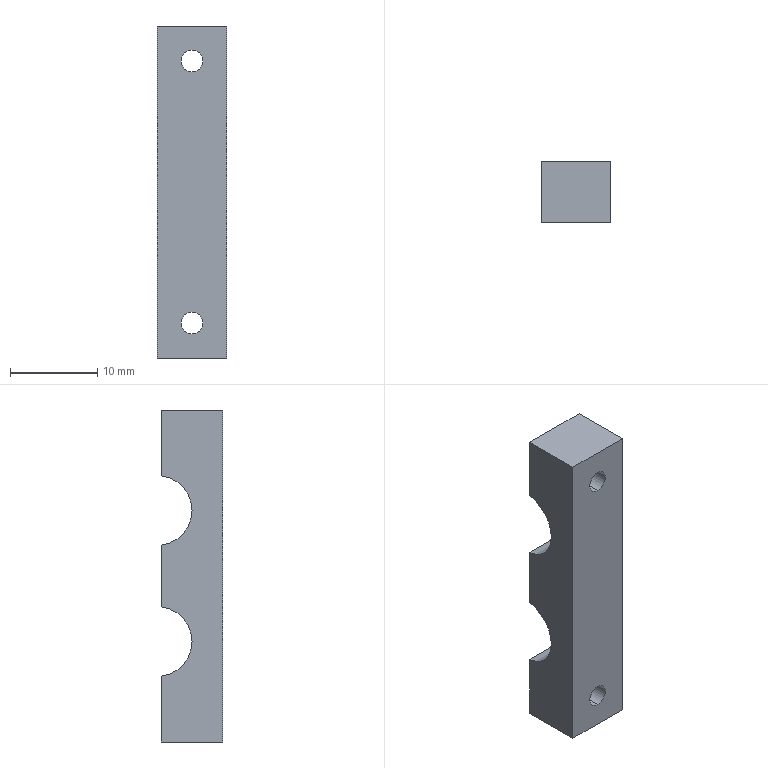Part | STEP file | 0246_217_Block | 1 solid | 14 faces | box 8 x 7 x 38 mm | volume 1721 mm3 | plane 8 | cylinder 6 | commonest cylinder face diameters 2.5 x4 8 x2
STEP:
#1=CARTESIAN_POINT('',(0.,0.,0.));
#2=DIRECTION('',(0.,0.,1.));
#3=DIRECTION('',(1.,0.,0.));
#4=AXIS2_PLACEMENT_3D('',#1,#2,#3);
#5=CARTESIAN_POINT('',(0.,0.,16.25));
#6=VERTEX_POINT('',#5);
#7=CARTESIAN_POINT('',(0.,7.,16.25));
#8=VERTEX_POINT('',#7);
#9=CARTESIAN_POINT('',(0.,7.,16.25));
#10=DIRECTION('',(0.,1.,0.));
#11=VECTOR('',#10,1.);
#12=LINE('',#9,#11);
#13=CARTESIAN_POINT('',(0.,7.,15.));
#14=DIRECTION('',(0.,1.,0.));
#15=DIRECTION('',(0.,0.,1.));
#16=AXIS2_PLACEMENT_3D('',#13,#14,#15);
#17=CYLINDRICAL_SURFACE('',#16,1.25);
#18=CARTESIAN_POINT('',(6.283,0.));
#19=DIRECTION('',(0.,1.));
#20=VECTOR('',#19,1.);
#21=LINE('',#18,#20);
#22=(GEOMETRIC_REPRESENTATION_CONTEXT(2)PARAMETRIC_REPRESENTATION_CONTEXT()REPRESENTATION_CONTEXT('',''));
#23=DEFINITIONAL_REPRESENTATION('',(#21),#22);
#24=PCURVE('',#17,#23);
#25=CARTESIAN_POINT('',(0.,7.,15.));
#26=DIRECTION('',(0.,1.,0.));
#27=DIRECTION('',(0.,0.,1.));
#28=AXIS2_PLACEMENT_3D('',#25,#26,#27);
#29=CYLINDRICAL_SURFACE('',#28,1.25);
#30=CARTESIAN_POINT('',(0.,0.));
#31=DIRECTION('',(0.,1.));
#32=VECTOR('',#31,1.);
#33=LINE('',#30,#32);
#34=(GEOMETRIC_REPRESENTATION_CONTEXT(2)PARAMETRIC_REPRESENTATION_CONTEXT()REPRESENTATION_CONTEXT('',''));
#35=DEFINITIONAL_REPRESENTATION('',(#33),#34);
#36=PCURVE('',#29,#35);
#37=SURFACE_CURVE('',#12,(#24,#36),.PCURVE_S1.);
#38=EDGE_CURVE('',#6,#8,#37,.T.);
#39=ORIENTED_EDGE('',*,*,#38,.T.);
#40=CARTESIAN_POINT('',(0.,7.,13.75));
#41=VERTEX_POINT('',#40);
#42=CARTESIAN_POINT('',(0.,7.,15.));
#43=DIRECTION('',(0.,1.,0.));
#44=DIRECTION('',(0.,0.,1.));
#45=AXIS2_PLACEMENT_3D('',#42,#43,#44);
#46=CIRCLE('',#45,1.25);
#47=CARTESIAN_POINT('',(0.,0.));
#48=DIRECTION('',(1.,0.));
#49=VECTOR('',#48,1.);
#50=LINE('',#47,#49);
#51=(GEOMETRIC_REPRESENTATION_CONTEXT(2)PARAMETRIC_REPRESENTATION_CONTEXT()REPRESENTATION_CONTEXT('',''));
#52=DEFINITIONAL_REPRESENTATION('',(#50),#51);
#53=PCURVE('',#17,#52);
#54=CARTESIAN_POINT('',(4.,7.,19.));
#55=DIRECTION('',(0.,-1.,0.));
#56=DIRECTION('',(0.,0.,-1.));
#57=AXIS2_PLACEMENT_3D('',#54,#55,#56);
#58=PLANE('',#57);
#59=CARTESIAN_POINT('',(2.75,-4.));
#60=CARTESIAN_POINT('',(2.75,-1.835));
#61=CARTESIAN_POINT('',(4.625,-2.917));
#62=CARTESIAN_POINT('',(6.5,-4.));
#63=CARTESIAN_POINT('',(4.625,-5.083));
#64=CARTESIAN_POINT('',(2.75,-6.165));
#65=CARTESIAN_POINT('',(2.75,-4.));
#66=(BOUNDED_CURVE()B_SPLINE_CURVE(2,(#59,#60,#61,#62,#63,#64,#65),.UNSPECIFIED.,.T.,.F.)B_SPLINE_CURVE_WITH_KNOTS((1,2,2,2,2,1),(-2.094,0.,2.094,4.189,6.283,8.378),.UNSPECIFIED.)CURVE()GEOMETRIC_REPRESENTATION_ITEM()RATIONAL_B_SPLINE_CURVE((1.,0.5,1.,0.5,1.,0.5,1.))REPRESENTATION_ITEM(''));
#67=(GEOMETRIC_REPRESENTATION_CONTEXT(2)PARAMETRIC_REPRESENTATION_CONTEXT()REPRESENTATION_CONTEXT('',''));
#68=DEFINITIONAL_REPRESENTATION('',(#66),#67);
#69=PCURVE('',#58,#68);
#70=SURFACE_CURVE('',#46,(#53,#69),.PCURVE_S1.);
#71=EDGE_CURVE('',#41,#8,#70,.T.);
#72=ORIENTED_EDGE('',*,*,#71,.F.);
#73=CARTESIAN_POINT('',(0.,0.,13.75));
#74=VERTEX_POINT('',#73);
#75=CARTESIAN_POINT('',(0.,7.,13.75));
#76=DIRECTION('',(0.,1.,0.));
#77=VECTOR('',#76,1.);
#78=LINE('',#75,#77);
#79=CARTESIAN_POINT('',(3.142,0.));
#80=DIRECTION('',(0.,1.));
#81=VECTOR('',#80,1.);
#82=LINE('',#79,#81);
#83=(GEOMETRIC_REPRESENTATION_CONTEXT(2)PARAMETRIC_REPRESENTATION_CONTEXT()REPRESENTATION_CONTEXT('',''));
#84=DEFINITIONAL_REPRESENTATION('',(#82),#83);
#85=PCURVE('',#17,#84);
#86=CARTESIAN_POINT('',(3.142,0.));
#87=DIRECTION('',(0.,1.));
#88=VECTOR('',#87,1.);
#89=LINE('',#86,#88);
#90=(GEOMETRIC_REPRESENTATION_CONTEXT(2)PARAMETRIC_REPRESENTATION_CONTEXT()REPRESENTATION_CONTEXT('',''));
#91=DEFINITIONAL_REPRESENTATION('',(#89),#90);
#92=PCURVE('',#29,#91);
#93=SURFACE_CURVE('',#78,(#85,#92),.PCURVE_S1.);
#94=EDGE_CURVE('',#74,#41,#93,.T.);
#95=ORIENTED_EDGE('',*,*,#94,.F.);
#96=CARTESIAN_POINT('',(0.,0.,15.));
#97=DIRECTION('',(0.,1.,0.));
#98=DIRECTION('',(0.,0.,1.));
#99=AXIS2_PLACEMENT_3D('',#96,#97,#98);
#100=CIRCLE('',#99,1.25);
#101=CARTESIAN_POINT('',(0.,-7.));
#102=DIRECTION('',(1.,0.));
#103=VECTOR('',#102,1.);
#104=LINE('',#101,#103);
#105=(GEOMETRIC_REPRESENTATION_CONTEXT(2)PARAMETRIC_REPRESENTATION_CONTEXT()REPRESENTATION_CONTEXT('',''));
#106=DEFINITIONAL_REPRESENTATION('',(#104),#105);
#107=PCURVE('',#17,#106);
#108=CARTESIAN_POINT('',(4.,0.,19.));
#109=DIRECTION('',(0.,1.,0.));
#110=DIRECTION('',(0.,0.,1.));
#111=AXIS2_PLACEMENT_3D('',#108,#109,#110);
#112=PLANE('',#111);
#113=CARTESIAN_POINT('',(-4.,-4.));
#114=DIRECTION('',(1.,0.));
#115=AXIS2_PLACEMENT_2D('',#113,#114);
#116=CIRCLE('',#115,1.25);
#117=(GEOMETRIC_REPRESENTATION_CONTEXT(2)PARAMETRIC_REPRESENTATION_CONTEXT()REPRESENTATION_CONTEXT('',''));
#118=DEFINITIONAL_REPRESENTATION('',(#116),#117);
#119=PCURVE('',#112,#118);
#120=SURFACE_CURVE('',#100,(#107,#119),.PCURVE_S1.);
#121=EDGE_CURVE('',#74,#6,#120,.T.);
#122=ORIENTED_EDGE('',*,*,#121,.T.);
#123=EDGE_LOOP('',(#39,#72,#95,#122));
#124=FACE_BOUND('',#123,.F.);
#125=ADVANCED_FACE('',(#124),#17,.F.);
#126=CARTESIAN_POINT('',(0.,0.,-13.75));
#127=VERTEX_POINT('',#126);
#128=CARTESIAN_POINT('',(0.,7.,-13.75));
#129=VERTEX_POINT('',#128);
#130=CARTESIAN_POINT('',(0.,7.,-13.75));
#131=DIRECTION('',(0.,1.,0.));
#132=VECTOR('',#131,1.);
#133=LINE('',#130,#132);
#134=CARTESIAN_POINT('',(0.,7.,-15.));
#135=DIRECTION('',(0.,1.,0.));
#136=DIRECTION('',(0.,0.,1.));
#137=AXIS2_PLACEMENT_3D('',#134,#135,#136);
#138=CYLINDRICAL_SURFACE('',#137,1.25);
#139=CARTESIAN_POINT('',(6.283,0.));
#140=DIRECTION('',(0.,1.));
#141=VECTOR('',#140,1.);
#142=LINE('',#139,#141);
#143=(GEOMETRIC_REPRESENTATION_CONTEXT(2)PARAMETRIC_REPRESENTATION_CONTEXT()REPRESENTATION_CONTEXT('',''));
#144=DEFINITIONAL_REPRESENTATION('',(#142),#143);
#145=PCURVE('',#138,#144);
#146=CARTESIAN_POINT('',(0.,7.,-15.));
#147=DIRECTION('',(0.,1.,0.));
#148=DIRECTION('',(0.,0.,1.));
#149=AXIS2_PLACEMENT_3D('',#146,#147,#148);
#150=CYLINDRICAL_SURFACE('',#149,1.25);
#151=CARTESIAN_POINT('',(0.,0.));
#152=DIRECTION('',(0.,1.));
#153=VECTOR('',#152,1.);
#154=LINE('',#151,#153);
#155=(GEOMETRIC_REPRESENTATION_CONTEXT(2)PARAMETRIC_REPRESENTATION_CONTEXT()REPRESENTATION_CONTEXT('',''));
#156=DEFINITIONAL_REPRESENTATION('',(#154),#155);
#157=PCURVE('',#150,#156);
#158=SURFACE_CURVE('',#133,(#145,#157),.PCURVE_S1.);
#159=EDGE_CURVE('',#127,#129,#158,.T.);
#160=ORIENTED_EDGE('',*,*,#159,.T.);
#161=CARTESIAN_POINT('',(0.,7.,-16.25));
#162=VERTEX_POINT('',#161);
#163=CARTESIAN_POINT('',(0.,7.,-15.));
#164=DIRECTION('',(0.,1.,0.));
#165=DIRECTION('',(0.,0.,1.));
#166=AXIS2_PLACEMENT_3D('',#163,#164,#165);
#167=CIRCLE('',#166,1.25);
#168=CARTESIAN_POINT('',(0.,0.));
#169=DIRECTION('',(1.,0.));
#170=VECTOR('',#169,1.);
#171=LINE('',#168,#170);
#172=(GEOMETRIC_REPRESENTATION_CONTEXT(2)PARAMETRIC_REPRESENTATION_CONTEXT()REPRESENTATION_CONTEXT('',''));
#173=DEFINITIONAL_REPRESENTATION('',(#171),#172);
#174=PCURVE('',#138,#173);
#175=CARTESIAN_POINT('',(4.,7.,-19.));
#176=DIRECTION('',(0.,-1.,0.));
#177=DIRECTION('',(0.,0.,-1.));
#178=AXIS2_PLACEMENT_3D('',#175,#176,#177);
#179=PLANE('',#178);
#180=CARTESIAN_POINT('',(-5.25,-4.));
#181=CARTESIAN_POINT('',(-5.25,-1.835));
#182=CARTESIAN_POINT('',(-3.375,-2.917));
#183=CARTESIAN_POINT('',(-1.5,-4.));
#184=CARTESIAN_POINT('',(-3.375,-5.083));
#185=CARTESIAN_POINT('',(-5.25,-6.165));
#186=CARTESIAN_POINT('',(-5.25,-4.));
#187=(BOUNDED_CURVE()B_SPLINE_CURVE(2,(#180,#181,#182,#183,#184,#185,#186),.UNSPECIFIED.,.T.,.F.)B_SPLINE_CURVE_WITH_KNOTS((1,2,2,2,2,1),(-2.094,0.,2.094,4.189,6.283,8.378),.UNSPECIFIED.)CURVE()GEOMETRIC_REPRESENTATION_ITEM()RATIONAL_B_SPLINE_CURVE((1.,0.5,1.,0.5,1.,0.5,1.))REPRESENTATION_ITEM(''));
#188=(GEOMETRIC_REPRESENTATION_CONTEXT(2)PARAMETRIC_REPRESENTATION_CONTEXT()REPRESENTATION_CONTEXT('',''));
#189=DEFINITIONAL_REPRESENTATION('',(#187),#188);
#190=PCURVE('',#179,#189);
#191=SURFACE_CURVE('',#167,(#174,#190),.PCURVE_S1.);
#192=EDGE_CURVE('',#162,#129,#191,.T.);
#193=ORIENTED_EDGE('',*,*,#192,.F.);
#194=CARTESIAN_POINT('',(0.,0.,-16.25));
#195=VERTEX_POINT('',#194);
#196=CARTESIAN_POINT('',(0.,7.,-16.25));
#197=DIRECTION('',(0.,1.,0.));
#198=VECTOR('',#197,1.);
#199=LINE('',#196,#198);
#200=CARTESIAN_POINT('',(3.142,0.));
#201=DIRECTION('',(0.,1.));
#202=VECTOR('',#201,1.);
#203=LINE('',#200,#202);
#204=(GEOMETRIC_REPRESENTATION_CONTEXT(2)PARAMETRIC_REPRESENTATION_CONTEXT()REPRESENTATION_CONTEXT('',''));
#205=DEFINITIONAL_REPRESENTATION('',(#203),#204);
#206=PCURVE('',#138,#205);
#207=CARTESIAN_POINT('',(3.142,0.));
#208=DIRECTION('',(0.,1.));
#209=VECTOR('',#208,1.);
#210=LINE('',#207,#209);
#211=(GEOMETRIC_REPRESENTATION_CONTEXT(2)PARAMETRIC_REPRESENTATION_CONTEXT()REPRESENTATION_CONTEXT('',''));
#212=DEFINITIONAL_REPRESENTATION('',(#210),#211);
#213=PCURVE('',#150,#212);
#214=SURFACE_CURVE('',#199,(#206,#213),.PCURVE_S1.);
#215=EDGE_CURVE('',#195,#162,#214,.T.);
#216=ORIENTED_EDGE('',*,*,#215,.F.);
#217=CARTESIAN_POINT('',(0.,0.,-15.));
#218=DIRECTION('',(0.,1.,0.));
#219=DIRECTION('',(0.,0.,1.));
#220=AXIS2_PLACEMENT_3D('',#217,#218,#219);
#221=CIRCLE('',#220,1.25);
#222=CARTESIAN_POINT('',(0.,-7.));
#223=DIRECTION('',(1.,0.));
#224=VECTOR('',#223,1.);
#225=LINE('',#222,#224);
#226=(GEOMETRIC_REPRESENTATION_CONTEXT(2)PARAMETRIC_REPRESENTATION_CONTEXT()REPRESENTATION_CONTEXT('',''));
#227=DEFINITIONAL_REPRESENTATION('',(#225),#226);
#228=PCURVE('',#138,#227);
#229=CARTESIAN_POINT('',(-34.,-4.));
#230=DIRECTION('',(1.,0.));
#231=AXIS2_PLACEMENT_2D('',#229,#230);
#232=CIRCLE('',#231,1.25);
#233=(GEOMETRIC_REPRESENTATION_CONTEXT(2)PARAMETRIC_REPRESENTATION_CONTEXT()REPRESENTATION_CONTEXT('',''));
#234=DEFINITIONAL_REPRESENTATION('',(#232),#233);
#235=PCURVE('',#112,#234);
#236=SURFACE_CURVE('',#221,(#228,#235),.PCURVE_S1.);
#237=EDGE_CURVE('',#195,#127,#236,.T.);
#238=ORIENTED_EDGE('',*,*,#237,.T.);
#239=EDGE_LOOP('',(#160,#193,#216,#238));
#240=FACE_BOUND('',#239,.F.);
#241=ADVANCED_FACE('',(#240),#138,.F.);
#242=CARTESIAN_POINT('',(-4.,7.,19.));
#243=VERTEX_POINT('',#242);
#244=CARTESIAN_POINT('',(-4.,0.,19.));
#245=VERTEX_POINT('',#244);
#246=CARTESIAN_POINT('',(-4.,0.,19.));
#247=DIRECTION('',(0.,-1.,0.));
#248=VECTOR('',#247,1.);
#249=LINE('',#246,#248);
#250=CARTESIAN_POINT('',(4.,0.,19.));
#251=DIRECTION('',(0.,0.,-1.));
#252=DIRECTION('',(-1.,0.,0.));
#253=AXIS2_PLACEMENT_3D('',#250,#251,#252);
#254=PLANE('',#253);
#255=CARTESIAN_POINT('',(8.,0.));
#256=DIRECTION('',(0.,-1.));
#257=VECTOR('',#256,1.);
#258=LINE('',#255,#257);
#259=(GEOMETRIC_REPRESENTATION_CONTEXT(2)PARAMETRIC_REPRESENTATION_CONTEXT()REPRESENTATION_CONTEXT('',''));
#260=DEFINITIONAL_REPRESENTATION('',(#258),#259);
#261=PCURVE('',#254,#260);
#262=CARTESIAN_POINT('',(-4.,7.5,7.5));
#263=DIRECTION('',(1.,0.,0.));
#264=DIRECTION('',(0.,0.,-1.));
#265=AXIS2_PLACEMENT_3D('',#262,#263,#264);
#266=PLANE('',#265);
#267=CARTESIAN_POINT('',(-11.5,-7.5));
#268=DIRECTION('',(0.,-1.));
#269=VECTOR('',#268,1.);
#270=LINE('',#267,#269);
#271=(GEOMETRIC_REPRESENTATION_CONTEXT(2)PARAMETRIC_REPRESENTATION_CONTEXT()REPRESENTATION_CONTEXT('',''));
#272=DEFINITIONAL_REPRESENTATION('',(#270),#271);
#273=PCURVE('',#266,#272);
#274=SURFACE_CURVE('',#249,(#261,#273),.PCURVE_S1.);
#275=EDGE_CURVE('',#243,#245,#274,.T.);
#276=ORIENTED_EDGE('',*,*,#275,.T.);
#277=CARTESIAN_POINT('',(4.,0.,19.));
#278=VERTEX_POINT('',#277);
#279=CARTESIAN_POINT('',(4.,0.,19.));
#280=DIRECTION('',(-1.,0.,0.));
#281=VECTOR('',#280,1.);
#282=LINE('',#279,#281);
#283=CARTESIAN_POINT('',(0.,0.));
#284=DIRECTION('',(1.,0.));
#285=VECTOR('',#284,1.);
#286=LINE('',#283,#285);
#287=(GEOMETRIC_REPRESENTATION_CONTEXT(2)PARAMETRIC_REPRESENTATION_CONTEXT()REPRESENTATION_CONTEXT('',''));
#288=DEFINITIONAL_REPRESENTATION('',(#286),#287);
#289=PCURVE('',#254,#288);
#290=CARTESIAN_POINT('',(0.,0.));
#291=DIRECTION('',(0.,-1.));
#292=VECTOR('',#291,1.);
#293=LINE('',#290,#292);
#294=(GEOMETRIC_REPRESENTATION_CONTEXT(2)PARAMETRIC_REPRESENTATION_CONTEXT()REPRESENTATION_CONTEXT('',''));
#295=DEFINITIONAL_REPRESENTATION('',(#293),#294);
#296=PCURVE('',#112,#295);
#297=SURFACE_CURVE('',#282,(#289,#296),.PCURVE_S1.);
#298=EDGE_CURVE('',#278,#245,#297,.T.);
#299=ORIENTED_EDGE('',*,*,#298,.F.);
#300=CARTESIAN_POINT('',(4.,7.,19.));
#301=VERTEX_POINT('',#300);
#302=CARTESIAN_POINT('',(4.,0.,19.));
#303=DIRECTION('',(0.,-1.,0.));
#304=VECTOR('',#303,1.);
#305=LINE('',#302,#304);
#306=CARTESIAN_POINT('',(0.,0.));
#307=DIRECTION('',(0.,-1.));
#308=VECTOR('',#307,1.);
#309=LINE('',#306,#308);
#310=(GEOMETRIC_REPRESENTATION_CONTEXT(2)PARAMETRIC_REPRESENTATION_CONTEXT()REPRESENTATION_CONTEXT('',''));
#311=DEFINITIONAL_REPRESENTATION('',(#309),#310);
#312=PCURVE('',#254,#311);
#313=CARTESIAN_POINT('',(4.,7.5,7.5));
#314=DIRECTION('',(1.,0.,0.));
#315=DIRECTION('',(0.,0.,-1.));
#316=AXIS2_PLACEMENT_3D('',#313,#314,#315);
#317=PLANE('',#316);
#318=CARTESIAN_POINT('',(-11.5,-7.5));
#319=DIRECTION('',(0.,-1.));
#320=VECTOR('',#319,1.);
#321=LINE('',#318,#320);
#322=(GEOMETRIC_REPRESENTATION_CONTEXT(2)PARAMETRIC_REPRESENTATION_CONTEXT()REPRESENTATION_CONTEXT('',''));
#323=DEFINITIONAL_REPRESENTATION('',(#321),#322);
#324=PCURVE('',#317,#323);
#325=SURFACE_CURVE('',#305,(#312,#324),.PCURVE_S1.);
#326=EDGE_CURVE('',#301,#278,#325,.T.);
#327=ORIENTED_EDGE('',*,*,#326,.F.);
#328=CARTESIAN_POINT('',(4.,7.,19.));
#329=DIRECTION('',(-1.,0.,0.));
#330=VECTOR('',#329,1.);
#331=LINE('',#328,#330);
#332=CARTESIAN_POINT('',(0.,7.));
#333=DIRECTION('',(1.,0.));
#334=VECTOR('',#333,1.);
#335=LINE('',#332,#334);
#336=(GEOMETRIC_REPRESENTATION_CONTEXT(2)PARAMETRIC_REPRESENTATION_CONTEXT()REPRESENTATION_CONTEXT('',''));
#337=DEFINITIONAL_REPRESENTATION('',(#335),#336);
#338=PCURVE('',#254,#337);
#339=CARTESIAN_POINT('',(0.,0.));
#340=DIRECTION('',(0.,-1.));
#341=VECTOR('',#340,1.);
#342=LINE('',#339,#341);
#343=(GEOMETRIC_REPRESENTATION_CONTEXT(2)PARAMETRIC_REPRESENTATION_CONTEXT()REPRESENTATION_CONTEXT('',''));
#344=DEFINITIONAL_REPRESENTATION('',(#342),#343);
#345=PCURVE('',#58,#344);
#346=SURFACE_CURVE('',#331,(#338,#345),.PCURVE_S1.);
#347=EDGE_CURVE('',#301,#243,#346,.T.);
#348=ORIENTED_EDGE('',*,*,#347,.T.);
#349=EDGE_LOOP('',(#276,#299,#327,#348));
#350=FACE_BOUND('',#349,.T.);
#351=ADVANCED_FACE('',(#350),#254,.F.);
#352=CARTESIAN_POINT('',(0.,0.,15.));
#353=DIRECTION('',(0.,1.,0.));
#354=DIRECTION('',(0.,0.,1.));
#355=AXIS2_PLACEMENT_3D('',#352,#353,#354);
#356=CIRCLE('',#355,1.25);
#357=CARTESIAN_POINT('',(-4.,-4.));
#358=DIRECTION('',(1.,0.));
#359=AXIS2_PLACEMENT_2D('',#357,#358);
#360=CIRCLE('',#359,1.25);
#361=(GEOMETRIC_REPRESENTATION_CONTEXT(2)PARAMETRIC_REPRESENTATION_CONTEXT()REPRESENTATION_CONTEXT('',''));
#362=DEFINITIONAL_REPRESENTATION('',(#360),#361);
#363=PCURVE('',#112,#362);
#364=CARTESIAN_POINT('',(0.,-7.));
#365=DIRECTION('',(1.,0.));
#366=VECTOR('',#365,1.);
#367=LINE('',#364,#366);
#368=(GEOMETRIC_REPRESENTATION_CONTEXT(2)PARAMETRIC_REPRESENTATION_CONTEXT()REPRESENTATION_CONTEXT('',''));
#369=DEFINITIONAL_REPRESENTATION('',(#367),#368);
#370=PCURVE('',#29,#369);
#371=SURFACE_CURVE('',#356,(#363,#370),.PCURVE_S1.);
#372=EDGE_CURVE('',#6,#74,#371,.T.);
#373=ORIENTED_EDGE('',*,*,#372,.T.);
#374=ORIENTED_EDGE('',*,*,#121,.T.);
#375=EDGE_LOOP('',(#373,#374));
#376=FACE_BOUND('',#375,.T.);
#377=CARTESIAN_POINT('',(0.,0.,-15.));
#378=DIRECTION('',(0.,1.,0.));
#379=DIRECTION('',(0.,0.,1.));
#380=AXIS2_PLACEMENT_3D('',#377,#378,#379);
#381=CIRCLE('',#380,1.25);
#382=CARTESIAN_POINT('',(-34.,-4.));
#383=DIRECTION('',(1.,0.));
#384=AXIS2_PLACEMENT_2D('',#382,#383);
#385=CIRCLE('',#384,1.25);
#386=(GEOMETRIC_REPRESENTATION_CONTEXT(2)PARAMETRIC_REPRESENTATION_CONTEXT()REPRESENTATION_CONTEXT('',''));
#387=DEFINITIONAL_REPRESENTATION('',(#385),#386);
#388=PCURVE('',#112,#387);
#389=CARTESIAN_POINT('',(0.,-7.));
#390=DIRECTION('',(1.,0.));
#391=VECTOR('',#390,1.);
#392=LINE('',#389,#391);
#393=(GEOMETRIC_REPRESENTATION_CONTEXT(2)PARAMETRIC_REPRESENTATION_CONTEXT()REPRESENTATION_CONTEXT('',''));
#394=DEFINITIONAL_REPRESENTATION('',(#392),#393);
#395=PCURVE('',#150,#394);
#396=SURFACE_CURVE('',#381,(#388,#395),.PCURVE_S1.);
#397=EDGE_CURVE('',#127,#195,#396,.T.);
#398=ORIENTED_EDGE('',*,*,#397,.T.);
#399=ORIENTED_EDGE('',*,*,#237,.T.);
#400=EDGE_LOOP('',(#398,#399));
#401=FACE_BOUND('',#400,.T.);
#402=CARTESIAN_POINT('',(-4.,0.,-19.));
#403=VERTEX_POINT('',#402);
#404=CARTESIAN_POINT('',(-4.,0.,19.));
#405=DIRECTION('',(0.,0.,-1.));
#406=VECTOR('',#405,1.);
#407=LINE('',#404,#406);
#408=CARTESIAN_POINT('',(0.,-8.));
#409=DIRECTION('',(-1.,0.));
#410=VECTOR('',#409,1.);
#411=LINE('',#408,#410);
#412=(GEOMETRIC_REPRESENTATION_CONTEXT(2)PARAMETRIC_REPRESENTATION_CONTEXT()REPRESENTATION_CONTEXT('',''));
#413=DEFINITIONAL_REPRESENTATION('',(#411),#412);
#414=PCURVE('',#112,#413);
#415=CARTESIAN_POINT('',(-11.5,-7.5));
#416=DIRECTION('',(1.,0.));
#417=VECTOR('',#416,1.);
#418=LINE('',#415,#417);
#419=(GEOMETRIC_REPRESENTATION_CONTEXT(2)PARAMETRIC_REPRESENTATION_CONTEXT()REPRESENTATION_CONTEXT('',''));
#420=DEFINITIONAL_REPRESENTATION('',(#418),#419);
#421=PCURVE('',#266,#420);
#422=SURFACE_CURVE('',#407,(#414,#421),.PCURVE_S1.);
#423=EDGE_CURVE('',#245,#403,#422,.T.);
#424=ORIENTED_EDGE('',*,*,#423,.T.);
#425=CARTESIAN_POINT('',(4.,0.,-19.));
#426=VERTEX_POINT('',#425);
#427=CARTESIAN_POINT('',(4.,0.,-19.));
#428=DIRECTION('',(-1.,0.,0.));
#429=VECTOR('',#428,1.);
#430=LINE('',#427,#429);
#431=CARTESIAN_POINT('',(-38.,0.));
#432=DIRECTION('',(0.,-1.));
#433=VECTOR('',#432,1.);
#434=LINE('',#431,#433);
#435=(GEOMETRIC_REPRESENTATION_CONTEXT(2)PARAMETRIC_REPRESENTATION_CONTEXT()REPRESENTATION_CONTEXT('',''));
#436=DEFINITIONAL_REPRESENTATION('',(#434),#435);
#437=PCURVE('',#112,#436);
#438=CARTESIAN_POINT('',(4.,0.,-19.));
#439=DIRECTION('',(0.,0.,1.));
#440=DIRECTION('',(1.,0.,0.));
#441=AXIS2_PLACEMENT_3D('',#438,#439,#440);
#442=PLANE('',#441);
#443=CARTESIAN_POINT('',(0.,0.));
#444=DIRECTION('',(-1.,0.));
#445=VECTOR('',#444,1.);
#446=LINE('',#443,#445);
#447=(GEOMETRIC_REPRESENTATION_CONTEXT(2)PARAMETRIC_REPRESENTATION_CONTEXT()REPRESENTATION_CONTEXT('',''));
#448=DEFINITIONAL_REPRESENTATION('',(#446),#447);
#449=PCURVE('',#442,#448);
#450=SURFACE_CURVE('',#430,(#437,#449),.PCURVE_S1.);
#451=EDGE_CURVE('',#426,#403,#450,.T.);
#452=ORIENTED_EDGE('',*,*,#451,.F.);
#453=CARTESIAN_POINT('',(4.,0.,19.));
#454=DIRECTION('',(0.,0.,-1.));
#455=VECTOR('',#454,1.);
#456=LINE('',#453,#455);
#457=CARTESIAN_POINT('',(0.,0.));
#458=DIRECTION('',(-1.,0.));
#459=VECTOR('',#458,1.);
#460=LINE('',#457,#459);
#461=(GEOMETRIC_REPRESENTATION_CONTEXT(2)PARAMETRIC_REPRESENTATION_CONTEXT()REPRESENTATION_CONTEXT('',''));
#462=DEFINITIONAL_REPRESENTATION('',(#460),#461);
#463=PCURVE('',#112,#462);
#464=CARTESIAN_POINT('',(-11.5,-7.5));
#465=DIRECTION('',(1.,0.));
#466=VECTOR('',#465,1.);
#467=LINE('',#464,#466);
#468=(GEOMETRIC_REPRESENTATION_CONTEXT(2)PARAMETRIC_REPRESENTATION_CONTEXT()REPRESENTATION_CONTEXT('',''));
#469=DEFINITIONAL_REPRESENTATION('',(#467),#468);
#470=PCURVE('',#317,#469);
#471=SURFACE_CURVE('',#456,(#463,#470),.PCURVE_S1.);
#472=EDGE_CURVE('',#278,#426,#471,.T.);
#473=ORIENTED_EDGE('',*,*,#472,.F.);
#474=ORIENTED_EDGE('',*,*,#298,.T.);
#475=EDGE_LOOP('',(#424,#452,#473,#474));
#476=FACE_BOUND('',#475,.T.);
#477=ADVANCED_FACE('',(#376,#401,#476),#112,.F.);
#478=CARTESIAN_POINT('',(-4.,7.,-19.));
#479=VERTEX_POINT('',#478);
#480=CARTESIAN_POINT('',(-4.,0.,-19.));
#481=DIRECTION('',(0.,1.,0.));
#482=VECTOR('',#481,1.);
#483=LINE('',#480,#482);
#484=CARTESIAN_POINT('',(-8.,0.));
#485=DIRECTION('',(0.,1.));
#486=VECTOR('',#485,1.);
#487=LINE('',#484,#486);
#488=(GEOMETRIC_REPRESENTATION_CONTEXT(2)PARAMETRIC_REPRESENTATION_CONTEXT()REPRESENTATION_CONTEXT('',''));
#489=DEFINITIONAL_REPRESENTATION('',(#487),#488);
#490=PCURVE('',#442,#489);
#491=CARTESIAN_POINT('',(26.5,-7.5));
#492=DIRECTION('',(0.,1.));
#493=VECTOR('',#492,1.);
#494=LINE('',#491,#493);
#495=(GEOMETRIC_REPRESENTATION_CONTEXT(2)PARAMETRIC_REPRESENTATION_CONTEXT()REPRESENTATION_CONTEXT('',''));
#496=DEFINITIONAL_REPRESENTATION('',(#494),#495);
#497=PCURVE('',#266,#496);
#498=SURFACE_CURVE('',#483,(#490,#497),.PCURVE_S1.);
#499=EDGE_CURVE('',#403,#479,#498,.T.);
#500=ORIENTED_EDGE('',*,*,#499,.T.);
#501=CARTESIAN_POINT('',(4.,7.,-19.));
#502=VERTEX_POINT('',#501);
#503=CARTESIAN_POINT('',(4.,7.,-19.));
#504=DIRECTION('',(-1.,0.,0.));
#505=VECTOR('',#504,1.);
#506=LINE('',#503,#505);
#507=CARTESIAN_POINT('',(0.,7.));
#508=DIRECTION('',(-1.,0.));
#509=VECTOR('',#508,1.);
#510=LINE('',#507,#509);
#511=(GEOMETRIC_REPRESENTATION_CONTEXT(2)PARAMETRIC_REPRESENTATION_CONTEXT()REPRESENTATION_CONTEXT('',''));
#512=DEFINITIONAL_REPRESENTATION('',(#510),#511);
#513=PCURVE('',#442,#512);
#514=CARTESIAN_POINT('',(0.,0.));
#515=DIRECTION('',(0.,-1.));
#516=VECTOR('',#515,1.);
#517=LINE('',#514,#516);
#518=(GEOMETRIC_REPRESENTATION_CONTEXT(2)PARAMETRIC_REPRESENTATION_CONTEXT()REPRESENTATION_CONTEXT('',''));
#519=DEFINITIONAL_REPRESENTATION('',(#517),#518);
#520=PCURVE('',#179,#519);
#521=SURFACE_CURVE('',#506,(#513,#520),.PCURVE_S1.);
#522=EDGE_CURVE('',#502,#479,#521,.T.);
#523=ORIENTED_EDGE('',*,*,#522,.F.);
#524=CARTESIAN_POINT('',(4.,0.,-19.));
#525=DIRECTION('',(0.,1.,0.));
#526=VECTOR('',#525,1.);
#527=LINE('',#524,#526);
#528=CARTESIAN_POINT('',(0.,0.));
#529=DIRECTION('',(0.,1.));
#530=VECTOR('',#529,1.);
#531=LINE('',#528,#530);
#532=(GEOMETRIC_REPRESENTATION_CONTEXT(2)PARAMETRIC_REPRESENTATION_CONTEXT()REPRESENTATION_CONTEXT('',''));
#533=DEFINITIONAL_REPRESENTATION('',(#531),#532);
#534=PCURVE('',#442,#533);
#535=CARTESIAN_POINT('',(26.5,-7.5));
#536=DIRECTION('',(0.,1.));
#537=VECTOR('',#536,1.);
#538=LINE('',#535,#537);
#539=(GEOMETRIC_REPRESENTATION_CONTEXT(2)PARAMETRIC_REPRESENTATION_CONTEXT()REPRESENTATION_CONTEXT('',''));
#540=DEFINITIONAL_REPRESENTATION('',(#538),#539);
#541=PCURVE('',#317,#540);
#542=SURFACE_CURVE('',#527,(#534,#541),.PCURVE_S1.);
#543=EDGE_CURVE('',#426,#502,#542,.T.);
#544=ORIENTED_EDGE('',*,*,#543,.F.);
#545=ORIENTED_EDGE('',*,*,#451,.T.);
#546=EDGE_LOOP('',(#500,#523,#544,#545));
#547=FACE_BOUND('',#546,.T.);
#548=ADVANCED_FACE('',(#547),#442,.F.);
#549=CARTESIAN_POINT('',(0.,7.,-15.));
#550=DIRECTION('',(0.,1.,0.));
#551=DIRECTION('',(0.,0.,1.));
#552=AXIS2_PLACEMENT_3D('',#549,#550,#551);
#553=CIRCLE('',#552,1.25);
#554=CARTESIAN_POINT('',(-5.25,-4.));
#555=CARTESIAN_POINT('',(-5.25,-1.835));
#556=CARTESIAN_POINT('',(-3.375,-2.917));
#557=CARTESIAN_POINT('',(-1.5,-4.));
#558=CARTESIAN_POINT('',(-3.375,-5.083));
#559=CARTESIAN_POINT('',(-5.25,-6.165));
#560=CARTESIAN_POINT('',(-5.25,-4.));
#561=(BOUNDED_CURVE()B_SPLINE_CURVE(2,(#554,#555,#556,#557,#558,#559,#560),.UNSPECIFIED.,.T.,.F.)B_SPLINE_CURVE_WITH_KNOTS((1,2,2,2,2,1),(-2.094,0.,2.094,4.189,6.283,8.378),.UNSPECIFIED.)CURVE()GEOMETRIC_REPRESENTATION_ITEM()RATIONAL_B_SPLINE_CURVE((1.,0.5,1.,0.5,1.,0.5,1.))REPRESENTATION_ITEM(''));
#562=(GEOMETRIC_REPRESENTATION_CONTEXT(2)PARAMETRIC_REPRESENTATION_CONTEXT()REPRESENTATION_CONTEXT('',''));
#563=DEFINITIONAL_REPRESENTATION('',(#561),#562);
#564=PCURVE('',#179,#563);
#565=CARTESIAN_POINT('',(0.,0.));
#566=DIRECTION('',(1.,0.));
#567=VECTOR('',#566,1.);
#568=LINE('',#565,#567);
#569=(GEOMETRIC_REPRESENTATION_CONTEXT(2)PARAMETRIC_REPRESENTATION_CONTEXT()REPRESENTATION_CONTEXT('',''));
#570=DEFINITIONAL_REPRESENTATION('',(#568),#569);
#571=PCURVE('',#150,#570);
#572=SURFACE_CURVE('',#553,(#564,#571),.PCURVE_S1.);
#573=EDGE_CURVE('',#129,#162,#572,.T.);
#574=ORIENTED_EDGE('',*,*,#573,.F.);
#575=ORIENTED_EDGE('',*,*,#192,.F.);
#576=EDGE_LOOP('',(#574,#575));
#577=FACE_BOUND('',#576,.T.);
#578=CARTESIAN_POINT('',(-4.,7.,-11.469));
#579=VERTEX_POINT('',#578);
#580=CARTESIAN_POINT('',(-4.,7.,-19.));
#581=DIRECTION('',(0.,0.,1.));
#582=VECTOR('',#581,1.);
#583=LINE('',#580,#582);
#584=CARTESIAN_POINT('',(0.,-8.));
#585=DIRECTION('',(-1.,0.));
#586=VECTOR('',#585,1.);
#587=LINE('',#584,#586);
#588=(GEOMETRIC_REPRESENTATION_CONTEXT(2)PARAMETRIC_REPRESENTATION_CONTEXT()REPRESENTATION_CONTEXT('',''));
#589=DEFINITIONAL_REPRESENTATION('',(#587),#588);
#590=PCURVE('',#179,#589);
#591=CARTESIAN_POINT('',(26.5,-0.5));
#592=DIRECTION('',(-1.,0.));
#593=VECTOR('',#592,1.);
#594=LINE('',#591,#593);
#595=(GEOMETRIC_REPRESENTATION_CONTEXT(2)PARAMETRIC_REPRESENTATION_CONTEXT()REPRESENTATION_CONTEXT('',''));
#596=DEFINITIONAL_REPRESENTATION('',(#594),#595);
#597=PCURVE('',#266,#596);
#598=SURFACE_CURVE('',#583,(#590,#597),.PCURVE_S1.);
#599=EDGE_CURVE('',#479,#579,#598,.T.);
#600=ORIENTED_EDGE('',*,*,#599,.T.);
#601=CARTESIAN_POINT('',(4.,7.,-11.469));
#602=VERTEX_POINT('',#601);
#603=CARTESIAN_POINT('',(4.,7.,-11.469));
#604=DIRECTION('',(-1.,0.,0.));
#605=VECTOR('',#604,1.);
#606=LINE('',#603,#605);
#607=CARTESIAN_POINT('',(-7.531,0.));
#608=DIRECTION('',(0.,-1.));
#609=VECTOR('',#608,1.);
#610=LINE('',#607,#609);
#611=(GEOMETRIC_REPRESENTATION_CONTEXT(2)PARAMETRIC_REPRESENTATION_CONTEXT()REPRESENTATION_CONTEXT('',''));
#612=DEFINITIONAL_REPRESENTATION('',(#610),#611);
#613=PCURVE('',#179,#612);
#614=CARTESIAN_POINT('',(4.,7.5,-7.5));
#615=DIRECTION('',(-1.,0.,0.));
#616=DIRECTION('',(0.,0.,1.));
#617=AXIS2_PLACEMENT_3D('',#614,#615,#616);
#618=CYLINDRICAL_SURFACE('',#617,4.);
#619=CARTESIAN_POINT('',(3.267,0.));
#620=DIRECTION('',(0.,1.));
#621=VECTOR('',#620,1.);
#622=LINE('',#619,#621);
#623=(GEOMETRIC_REPRESENTATION_CONTEXT(2)PARAMETRIC_REPRESENTATION_CONTEXT()REPRESENTATION_CONTEXT('',''));
#624=DEFINITIONAL_REPRESENTATION('',(#622),#623);
#625=PCURVE('',#618,#624);
#626=SURFACE_CURVE('',#606,(#613,#625),.PCURVE_S1.);
#627=EDGE_CURVE('',#602,#579,#626,.T.);
#628=ORIENTED_EDGE('',*,*,#627,.F.);
#629=CARTESIAN_POINT('',(4.,7.,-19.));
#630=DIRECTION('',(0.,0.,1.));
#631=VECTOR('',#630,1.);
#632=LINE('',#629,#631);
#633=CARTESIAN_POINT('',(0.,0.));
#634=DIRECTION('',(-1.,0.));
#635=VECTOR('',#634,1.);
#636=LINE('',#633,#635);
#637=(GEOMETRIC_REPRESENTATION_CONTEXT(2)PARAMETRIC_REPRESENTATION_CONTEXT()REPRESENTATION_CONTEXT('',''));
#638=DEFINITIONAL_REPRESENTATION('',(#636),#637);
#639=PCURVE('',#179,#638);
#640=CARTESIAN_POINT('',(26.5,-0.5));
#641=DIRECTION('',(-1.,0.));
#642=VECTOR('',#641,1.);
#643=LINE('',#640,#642);
#644=(GEOMETRIC_REPRESENTATION_CONTEXT(2)PARAMETRIC_REPRESENTATION_CONTEXT()REPRESENTATION_CONTEXT('',''));
#645=DEFINITIONAL_REPRESENTATION('',(#643),#644);
#646=PCURVE('',#317,#645);
#647=SURFACE_CURVE('',#632,(#639,#646),.PCURVE_S1.);
#648=EDGE_CURVE('',#502,#602,#647,.T.);
#649=ORIENTED_EDGE('',*,*,#648,.F.);
#650=ORIENTED_EDGE('',*,*,#522,.T.);
#651=EDGE_LOOP('',(#600,#628,#649,#650));
#652=FACE_BOUND('',#651,.T.);
#653=ADVANCED_FACE('',(#577,#652),#179,.F.);
#654=ORIENTED_EDGE('',*,*,#627,.F.);
#655=CARTESIAN_POINT('',(4.,7.,-3.531));
#656=VERTEX_POINT('',#655);
#657=CARTESIAN_POINT('',(4.,7.5,-7.5));
#658=DIRECTION('',(-1.,0.,0.));
#659=DIRECTION('',(0.,0.,-1.));
#660=AXIS2_PLACEMENT_3D('',#657,#658,#659);
#661=CIRCLE('',#660,4.);
#662=CARTESIAN_POINT('',(3.142,0.));
#663=DIRECTION('',(1.,0.));
#664=VECTOR('',#663,1.);
#665=LINE('',#662,#664);
#666=(GEOMETRIC_REPRESENTATION_CONTEXT(2)PARAMETRIC_REPRESENTATION_CONTEXT()REPRESENTATION_CONTEXT('',''));
#667=DEFINITIONAL_REPRESENTATION('',(#665),#666);
#668=PCURVE('',#618,#667);
#669=CARTESIAN_POINT('',(19.,0.));
#670=CARTESIAN_POINT('',(19.,-6.928));
#671=CARTESIAN_POINT('',(13.,-3.464));
#672=CARTESIAN_POINT('',(7.,0.));
#673=CARTESIAN_POINT('',(13.,3.464));
#674=CARTESIAN_POINT('',(19.,6.928));
#675=CARTESIAN_POINT('',(19.,0.));
#676=(BOUNDED_CURVE()B_SPLINE_CURVE(2,(#669,#670,#671,#672,#673,#674,#675),.UNSPECIFIED.,.T.,.F.)B_SPLINE_CURVE_WITH_KNOTS((1,2,2,2,2,1),(-2.094,0.,2.094,4.189,6.283,8.378),.UNSPECIFIED.)CURVE()GEOMETRIC_REPRESENTATION_ITEM()RATIONAL_B_SPLINE_CURVE((1.,0.5,1.,0.5,1.,0.5,1.))REPRESENTATION_ITEM(''));
#677=(GEOMETRIC_REPRESENTATION_CONTEXT(2)PARAMETRIC_REPRESENTATION_CONTEXT()REPRESENTATION_CONTEXT('',''));
#678=DEFINITIONAL_REPRESENTATION('',(#676),#677);
#679=PCURVE('',#317,#678);
#680=SURFACE_CURVE('',#661,(#668,#679),.PCURVE_S1.);
#681=EDGE_CURVE('',#602,#656,#680,.T.);
#682=ORIENTED_EDGE('',*,*,#681,.T.);
#683=CARTESIAN_POINT('',(-4.,7.,-3.531));
#684=VERTEX_POINT('',#683);
#685=CARTESIAN_POINT('',(4.,7.,-3.531));
#686=DIRECTION('',(-1.,0.,0.));
#687=VECTOR('',#686,1.);
#688=LINE('',#685,#687);
#689=CARTESIAN_POINT('',(6.158,0.));
#690=DIRECTION('',(0.,1.));
#691=VECTOR('',#690,1.);
#692=LINE('',#689,#691);
#693=(GEOMETRIC_REPRESENTATION_CONTEXT(2)PARAMETRIC_REPRESENTATION_CONTEXT()REPRESENTATION_CONTEXT('',''));
#694=DEFINITIONAL_REPRESENTATION('',(#692),#693);
#695=PCURVE('',#618,#694);
#696=CARTESIAN_POINT('',(4.,7.,3.531));
#697=DIRECTION('',(0.,-1.,0.));
#698=DIRECTION('',(0.,0.,-1.));
#699=AXIS2_PLACEMENT_3D('',#696,#697,#698);
#700=PLANE('',#699);
#701=CARTESIAN_POINT('',(7.063,0.));
#702=DIRECTION('',(0.,-1.));
#703=VECTOR('',#702,1.);
#704=LINE('',#701,#703);
#705=(GEOMETRIC_REPRESENTATION_CONTEXT(2)PARAMETRIC_REPRESENTATION_CONTEXT()REPRESENTATION_CONTEXT('',''));
#706=DEFINITIONAL_REPRESENTATION('',(#704),#705);
#707=PCURVE('',#700,#706);
#708=SURFACE_CURVE('',#688,(#695,#707),.PCURVE_S1.);
#709=EDGE_CURVE('',#656,#684,#708,.T.);
#710=ORIENTED_EDGE('',*,*,#709,.T.);
#711=CARTESIAN_POINT('',(-4.,7.5,-7.5));
#712=DIRECTION('',(-1.,0.,0.));
#713=DIRECTION('',(0.,0.,-1.));
#714=AXIS2_PLACEMENT_3D('',#711,#712,#713);
#715=CIRCLE('',#714,4.);
#716=CARTESIAN_POINT('',(3.142,8.));
#717=DIRECTION('',(1.,0.));
#718=VECTOR('',#717,1.);
#719=LINE('',#716,#718);
#720=(GEOMETRIC_REPRESENTATION_CONTEXT(2)PARAMETRIC_REPRESENTATION_CONTEXT()REPRESENTATION_CONTEXT('',''));
#721=DEFINITIONAL_REPRESENTATION('',(#719),#720);
#722=PCURVE('',#618,#721);
#723=CARTESIAN_POINT('',(19.,0.));
#724=CARTESIAN_POINT('',(19.,-6.928));
#725=CARTESIAN_POINT('',(13.,-3.464));
#726=CARTESIAN_POINT('',(7.,0.));
#727=CARTESIAN_POINT('',(13.,3.464));
#728=CARTESIAN_POINT('',(19.,6.928));
#729=CARTESIAN_POINT('',(19.,0.));
#730=(BOUNDED_CURVE()B_SPLINE_CURVE(2,(#723,#724,#725,#726,#727,#728,#729),.UNSPECIFIED.,.T.,.F.)B_SPLINE_CURVE_WITH_KNOTS((1,2,2,2,2,1),(-2.094,0.,2.094,4.189,6.283,8.378),.UNSPECIFIED.)CURVE()GEOMETRIC_REPRESENTATION_ITEM()RATIONAL_B_SPLINE_CURVE((1.,0.5,1.,0.5,1.,0.5,1.))REPRESENTATION_ITEM(''));
#731=(GEOMETRIC_REPRESENTATION_CONTEXT(2)PARAMETRIC_REPRESENTATION_CONTEXT()REPRESENTATION_CONTEXT('',''));
#732=DEFINITIONAL_REPRESENTATION('',(#730),#731);
#733=PCURVE('',#266,#732);
#734=SURFACE_CURVE('',#715,(#722,#733),.PCURVE_S1.);
#735=EDGE_CURVE('',#579,#684,#734,.T.);
#736=ORIENTED_EDGE('',*,*,#735,.F.);
#737=EDGE_LOOP('',(#654,#682,#710,#736));
#738=FACE_BOUND('',#737,.F.);
#739=ADVANCED_FACE('',(#738),#618,.F.);
#740=CARTESIAN_POINT('',(-4.,7.,3.531));
#741=VERTEX_POINT('',#740);
#742=CARTESIAN_POINT('',(-4.,7.,3.531));
#743=DIRECTION('',(0.,0.,1.));
#744=VECTOR('',#743,1.);
#745=LINE('',#742,#744);
#746=CARTESIAN_POINT('',(0.,-8.));
#747=DIRECTION('',(-1.,0.));
#748=VECTOR('',#747,1.);
#749=LINE('',#746,#748);
#750=(GEOMETRIC_REPRESENTATION_CONTEXT(2)PARAMETRIC_REPRESENTATION_CONTEXT()REPRESENTATION_CONTEXT('',''));
#751=DEFINITIONAL_REPRESENTATION('',(#749),#750);
#752=PCURVE('',#700,#751);
#753=CARTESIAN_POINT('',(3.969,-0.5));
#754=DIRECTION('',(-1.,0.));
#755=VECTOR('',#754,1.);
#756=LINE('',#753,#755);
#757=(GEOMETRIC_REPRESENTATION_CONTEXT(2)PARAMETRIC_REPRESENTATION_CONTEXT()REPRESENTATION_CONTEXT('',''));
#758=DEFINITIONAL_REPRESENTATION('',(#756),#757);
#759=PCURVE('',#266,#758);
#760=SURFACE_CURVE('',#745,(#752,#759),.PCURVE_S1.);
#761=EDGE_CURVE('',#684,#741,#760,.T.);
#762=ORIENTED_EDGE('',*,*,#761,.T.);
#763=CARTESIAN_POINT('',(4.,7.,3.531));
#764=VERTEX_POINT('',#763);
#765=CARTESIAN_POINT('',(4.,7.,3.531));
#766=DIRECTION('',(-1.,0.,0.));
#767=VECTOR('',#766,1.);
#768=LINE('',#765,#767);
#769=CARTESIAN_POINT('',(0.,0.));
#770=DIRECTION('',(0.,-1.));
#771=VECTOR('',#770,1.);
#772=LINE('',#769,#771);
#773=(GEOMETRIC_REPRESENTATION_CONTEXT(2)PARAMETRIC_REPRESENTATION_CONTEXT()REPRESENTATION_CONTEXT('',''));
#774=DEFINITIONAL_REPRESENTATION('',(#772),#773);
#775=PCURVE('',#700,#774);
#776=CARTESIAN_POINT('',(4.,7.5,7.5));
#777=DIRECTION('',(-1.,0.,0.));
#778=DIRECTION('',(0.,0.,1.));
#779=AXIS2_PLACEMENT_3D('',#776,#777,#778);
#780=CYLINDRICAL_SURFACE('',#779,4.);
#781=CARTESIAN_POINT('',(3.267,0.));
#782=DIRECTION('',(0.,1.));
#783=VECTOR('',#782,1.);
#784=LINE('',#781,#783);
#785=(GEOMETRIC_REPRESENTATION_CONTEXT(2)PARAMETRIC_REPRESENTATION_CONTEXT()REPRESENTATION_CONTEXT('',''));
#786=DEFINITIONAL_REPRESENTATION('',(#784),#785);
#787=PCURVE('',#780,#786);
#788=SURFACE_CURVE('',#768,(#775,#787),.PCURVE_S1.);
#789=EDGE_CURVE('',#764,#741,#788,.T.);
#790=ORIENTED_EDGE('',*,*,#789,.F.);
#791=CARTESIAN_POINT('',(4.,7.,3.531));
#792=DIRECTION('',(0.,0.,1.));
#793=VECTOR('',#792,1.);
#794=LINE('',#791,#793);
#795=CARTESIAN_POINT('',(0.,0.));
#796=DIRECTION('',(-1.,0.));
#797=VECTOR('',#796,1.);
#798=LINE('',#795,#797);
#799=(GEOMETRIC_REPRESENTATION_CONTEXT(2)PARAMETRIC_REPRESENTATION_CONTEXT()REPRESENTATION_CONTEXT('',''));
#800=DEFINITIONAL_REPRESENTATION('',(#798),#799);
#801=PCURVE('',#700,#800);
#802=CARTESIAN_POINT('',(3.969,-0.5));
#803=DIRECTION('',(-1.,0.));
#804=VECTOR('',#803,1.);
#805=LINE('',#802,#804);
#806=(GEOMETRIC_REPRESENTATION_CONTEXT(2)PARAMETRIC_REPRESENTATION_CONTEXT()REPRESENTATION_CONTEXT('',''));
#807=DEFINITIONAL_REPRESENTATION('',(#805),#806);
#808=PCURVE('',#317,#807);
#809=SURFACE_CURVE('',#794,(#801,#808),.PCURVE_S1.);
#810=EDGE_CURVE('',#656,#764,#809,.T.);
#811=ORIENTED_EDGE('',*,*,#810,.F.);
#812=ORIENTED_EDGE('',*,*,#709,.T.);
#813=EDGE_LOOP('',(#762,#790,#811,#812));
#814=FACE_BOUND('',#813,.T.);
#815=ADVANCED_FACE('',(#814),#700,.F.);
#816=ORIENTED_EDGE('',*,*,#789,.F.);
#817=CARTESIAN_POINT('',(4.,7.,11.469));
#818=VERTEX_POINT('',#817);
#819=CARTESIAN_POINT('',(4.,7.5,7.5));
#820=DIRECTION('',(-1.,0.,0.));
#821=DIRECTION('',(0.,0.,-1.));
#822=AXIS2_PLACEMENT_3D('',#819,#820,#821);
#823=CIRCLE('',#822,4.);
#824=CARTESIAN_POINT('',(3.142,0.));
#825=DIRECTION('',(1.,0.));
#826=VECTOR('',#825,1.);
#827=LINE('',#824,#826);
#828=(GEOMETRIC_REPRESENTATION_CONTEXT(2)PARAMETRIC_REPRESENTATION_CONTEXT()REPRESENTATION_CONTEXT('',''));
#829=DEFINITIONAL_REPRESENTATION('',(#827),#828);
#830=PCURVE('',#780,#829);
#831=CARTESIAN_POINT('',(4.,0.));
#832=CARTESIAN_POINT('',(4.,-6.928));
#833=CARTESIAN_POINT('',(-2.,-3.464));
#834=CARTESIAN_POINT('',(-8.,0.));
#835=CARTESIAN_POINT('',(-2.,3.464));
#836=CARTESIAN_POINT('',(4.,6.928));
#837=CARTESIAN_POINT('',(4.,0.));
#838=(BOUNDED_CURVE()B_SPLINE_CURVE(2,(#831,#832,#833,#834,#835,#836,#837),.UNSPECIFIED.,.T.,.F.)B_SPLINE_CURVE_WITH_KNOTS((1,2,2,2,2,1),(-2.094,0.,2.094,4.189,6.283,8.378),.UNSPECIFIED.)CURVE()GEOMETRIC_REPRESENTATION_ITEM()RATIONAL_B_SPLINE_CURVE((1.,0.5,1.,0.5,1.,0.5,1.))REPRESENTATION_ITEM(''));
#839=(GEOMETRIC_REPRESENTATION_CONTEXT(2)PARAMETRIC_REPRESENTATION_CONTEXT()REPRESENTATION_CONTEXT('',''));
#840=DEFINITIONAL_REPRESENTATION('',(#838),#839);
#841=PCURVE('',#317,#840);
#842=SURFACE_CURVE('',#823,(#830,#841),.PCURVE_S1.);
#843=EDGE_CURVE('',#764,#818,#842,.T.);
#844=ORIENTED_EDGE('',*,*,#843,.T.);
#845=CARTESIAN_POINT('',(-4.,7.,11.469));
#846=VERTEX_POINT('',#845);
#847=CARTESIAN_POINT('',(4.,7.,11.469));
#848=DIRECTION('',(-1.,0.,0.));
#849=VECTOR('',#848,1.);
#850=LINE('',#847,#849);
#851=CARTESIAN_POINT('',(6.158,0.));
#852=DIRECTION('',(0.,1.));
#853=VECTOR('',#852,1.);
#854=LINE('',#851,#853);
#855=(GEOMETRIC_REPRESENTATION_CONTEXT(2)PARAMETRIC_REPRESENTATION_CONTEXT()REPRESENTATION_CONTEXT('',''));
#856=DEFINITIONAL_REPRESENTATION('',(#854),#855);
#857=PCURVE('',#780,#856);
#858=CARTESIAN_POINT('',(7.531,0.));
#859=DIRECTION('',(0.,-1.));
#860=VECTOR('',#859,1.);
#861=LINE('',#858,#860);
#862=(GEOMETRIC_REPRESENTATION_CONTEXT(2)PARAMETRIC_REPRESENTATION_CONTEXT()REPRESENTATION_CONTEXT('',''));
#863=DEFINITIONAL_REPRESENTATION('',(#861),#862);
#864=PCURVE('',#58,#863);
#865=SURFACE_CURVE('',#850,(#857,#864),.PCURVE_S1.);
#866=EDGE_CURVE('',#818,#846,#865,.T.);
#867=ORIENTED_EDGE('',*,*,#866,.T.);
#868=CARTESIAN_POINT('',(-4.,7.5,7.5));
#869=DIRECTION('',(-1.,0.,0.));
#870=DIRECTION('',(0.,0.,-1.));
#871=AXIS2_PLACEMENT_3D('',#868,#869,#870);
#872=CIRCLE('',#871,4.);
#873=CARTESIAN_POINT('',(3.142,8.));
#874=DIRECTION('',(1.,0.));
#875=VECTOR('',#874,1.);
#876=LINE('',#873,#875);
#877=(GEOMETRIC_REPRESENTATION_CONTEXT(2)PARAMETRIC_REPRESENTATION_CONTEXT()REPRESENTATION_CONTEXT('',''));
#878=DEFINITIONAL_REPRESENTATION('',(#876),#877);
#879=PCURVE('',#780,#878);
#880=CARTESIAN_POINT('',(4.,0.));
#881=CARTESIAN_POINT('',(4.,-6.928));
#882=CARTESIAN_POINT('',(-2.,-3.464));
#883=CARTESIAN_POINT('',(-8.,0.));
#884=CARTESIAN_POINT('',(-2.,3.464));
#885=CARTESIAN_POINT('',(4.,6.928));
#886=CARTESIAN_POINT('',(4.,0.));
#887=(BOUNDED_CURVE()B_SPLINE_CURVE(2,(#880,#881,#882,#883,#884,#885,#886),.UNSPECIFIED.,.T.,.F.)B_SPLINE_CURVE_WITH_KNOTS((1,2,2,2,2,1),(-2.094,0.,2.094,4.189,6.283,8.378),.UNSPECIFIED.)CURVE()GEOMETRIC_REPRESENTATION_ITEM()RATIONAL_B_SPLINE_CURVE((1.,0.5,1.,0.5,1.,0.5,1.))REPRESENTATION_ITEM(''));
#888=(GEOMETRIC_REPRESENTATION_CONTEXT(2)PARAMETRIC_REPRESENTATION_CONTEXT()REPRESENTATION_CONTEXT('',''));
#889=DEFINITIONAL_REPRESENTATION('',(#887),#888);
#890=PCURVE('',#266,#889);
#891=SURFACE_CURVE('',#872,(#879,#890),.PCURVE_S1.);
#892=EDGE_CURVE('',#741,#846,#891,.T.);
#893=ORIENTED_EDGE('',*,*,#892,.F.);
#894=EDGE_LOOP('',(#816,#844,#867,#893));
#895=FACE_BOUND('',#894,.F.);
#896=ADVANCED_FACE('',(#895),#780,.F.);
#897=CARTESIAN_POINT('',(0.,7.,15.));
#898=DIRECTION('',(0.,1.,0.));
#899=DIRECTION('',(0.,0.,1.));
#900=AXIS2_PLACEMENT_3D('',#897,#898,#899);
#901=CIRCLE('',#900,1.25);
#902=CARTESIAN_POINT('',(2.75,-4.));
#903=CARTESIAN_POINT('',(2.75,-1.835));
#904=CARTESIAN_POINT('',(4.625,-2.917));
#905=CARTESIAN_POINT('',(6.5,-4.));
#906=CARTESIAN_POINT('',(4.625,-5.083));
#907=CARTESIAN_POINT('',(2.75,-6.165));
#908=CARTESIAN_POINT('',(2.75,-4.));
#909=(BOUNDED_CURVE()B_SPLINE_CURVE(2,(#902,#903,#904,#905,#906,#907,#908),.UNSPECIFIED.,.T.,.F.)B_SPLINE_CURVE_WITH_KNOTS((1,2,2,2,2,1),(-2.094,0.,2.094,4.189,6.283,8.378),.UNSPECIFIED.)CURVE()GEOMETRIC_REPRESENTATION_ITEM()RATIONAL_B_SPLINE_CURVE((1.,0.5,1.,0.5,1.,0.5,1.))REPRESENTATION_ITEM(''));
#910=(GEOMETRIC_REPRESENTATION_CONTEXT(2)PARAMETRIC_REPRESENTATION_CONTEXT()REPRESENTATION_CONTEXT('',''));
#911=DEFINITIONAL_REPRESENTATION('',(#909),#910);
#912=PCURVE('',#58,#911);
#913=CARTESIAN_POINT('',(0.,0.));
#914=DIRECTION('',(1.,0.));
#915=VECTOR('',#914,1.);
#916=LINE('',#913,#915);
#917=(GEOMETRIC_REPRESENTATION_CONTEXT(2)PARAMETRIC_REPRESENTATION_CONTEXT()REPRESENTATION_CONTEXT('',''));
#918=DEFINITIONAL_REPRESENTATION('',(#916),#917);
#919=PCURVE('',#29,#918);
#920=SURFACE_CURVE('',#901,(#912,#919),.PCURVE_S1.);
#921=EDGE_CURVE('',#8,#41,#920,.T.);
#922=ORIENTED_EDGE('',*,*,#921,.F.);
#923=ORIENTED_EDGE('',*,*,#71,.F.);
#924=EDGE_LOOP('',(#922,#923));
#925=FACE_BOUND('',#924,.T.);
#926=CARTESIAN_POINT('',(-4.,7.,19.));
#927=DIRECTION('',(0.,0.,1.));
#928=VECTOR('',#927,1.);
#929=LINE('',#926,#928);
#930=CARTESIAN_POINT('',(0.,-8.));
#931=DIRECTION('',(-1.,0.));
#932=VECTOR('',#931,1.);
#933=LINE('',#930,#932);
#934=(GEOMETRIC_REPRESENTATION_CONTEXT(2)PARAMETRIC_REPRESENTATION_CONTEXT()REPRESENTATION_CONTEXT('',''));
#935=DEFINITIONAL_REPRESENTATION('',(#933),#934);
#936=PCURVE('',#58,#935);
#937=CARTESIAN_POINT('',(-11.5,-0.5));
#938=DIRECTION('',(-1.,0.));
#939=VECTOR('',#938,1.);
#940=LINE('',#937,#939);
#941=(GEOMETRIC_REPRESENTATION_CONTEXT(2)PARAMETRIC_REPRESENTATION_CONTEXT()REPRESENTATION_CONTEXT('',''));
#942=DEFINITIONAL_REPRESENTATION('',(#940),#941);
#943=PCURVE('',#266,#942);
#944=SURFACE_CURVE('',#929,(#936,#943),.PCURVE_S1.);
#945=EDGE_CURVE('',#846,#243,#944,.T.);
#946=ORIENTED_EDGE('',*,*,#945,.T.);
#947=ORIENTED_EDGE('',*,*,#347,.F.);
#948=CARTESIAN_POINT('',(4.,7.,19.));
#949=DIRECTION('',(0.,0.,1.));
#950=VECTOR('',#949,1.);
#951=LINE('',#948,#950);
#952=CARTESIAN_POINT('',(0.,0.));
#953=DIRECTION('',(-1.,0.));
#954=VECTOR('',#953,1.);
#955=LINE('',#952,#954);
#956=(GEOMETRIC_REPRESENTATION_CONTEXT(2)PARAMETRIC_REPRESENTATION_CONTEXT()REPRESENTATION_CONTEXT('',''));
#957=DEFINITIONAL_REPRESENTATION('',(#955),#956);
#958=PCURVE('',#58,#957);
#959=CARTESIAN_POINT('',(-11.5,-0.5));
#960=DIRECTION('',(-1.,0.));
#961=VECTOR('',#960,1.);
#962=LINE('',#959,#961);
#963=(GEOMETRIC_REPRESENTATION_CONTEXT(2)PARAMETRIC_REPRESENTATION_CONTEXT()REPRESENTATION_CONTEXT('',''));
#964=DEFINITIONAL_REPRESENTATION('',(#962),#963);
#965=PCURVE('',#317,#964);
#966=SURFACE_CURVE('',#951,(#958,#965),.PCURVE_S1.);
#967=EDGE_CURVE('',#818,#301,#966,.T.);
#968=ORIENTED_EDGE('',*,*,#967,.F.);
#969=ORIENTED_EDGE('',*,*,#866,.T.);
#970=EDGE_LOOP('',(#946,#947,#968,#969));
#971=FACE_BOUND('',#970,.T.);
#972=ADVANCED_FACE('',(#925,#971),#58,.F.);
#973=ORIENTED_EDGE('',*,*,#326,.T.);
#974=ORIENTED_EDGE('',*,*,#472,.T.);
#975=ORIENTED_EDGE('',*,*,#543,.T.);
#976=ORIENTED_EDGE('',*,*,#648,.T.);
#977=ORIENTED_EDGE('',*,*,#681,.T.);
#978=ORIENTED_EDGE('',*,*,#810,.T.);
#979=ORIENTED_EDGE('',*,*,#843,.T.);
#980=ORIENTED_EDGE('',*,*,#967,.T.);
#981=EDGE_LOOP('',(#973,#974,#975,#976,#977,#978,#979,#980));
#982=FACE_BOUND('',#981,.T.);
#983=ADVANCED_FACE('',(#982),#317,.T.);
#984=ORIENTED_EDGE('',*,*,#275,.F.);
#985=ORIENTED_EDGE('',*,*,#945,.F.);
#986=ORIENTED_EDGE('',*,*,#892,.F.);
#987=ORIENTED_EDGE('',*,*,#761,.F.);
#988=ORIENTED_EDGE('',*,*,#735,.F.);
#989=ORIENTED_EDGE('',*,*,#599,.F.);
#990=ORIENTED_EDGE('',*,*,#499,.F.);
#991=ORIENTED_EDGE('',*,*,#423,.F.);
#992=EDGE_LOOP('',(#984,#985,#986,#987,#988,#989,#990,#991));
#993=FACE_BOUND('',#992,.T.);
#994=ADVANCED_FACE('',(#993),#266,.F.);
#995=ORIENTED_EDGE('',*,*,#573,.F.);
#996=ORIENTED_EDGE('',*,*,#159,.F.);
#997=ORIENTED_EDGE('',*,*,#397,.T.);
#998=ORIENTED_EDGE('',*,*,#215,.T.);
#999=EDGE_LOOP('',(#995,#996,#997,#998));
#1000=FACE_BOUND('',#999,.F.);
#1001=ADVANCED_FACE('',(#1000),#150,.F.);
#1002=ORIENTED_EDGE('',*,*,#921,.F.);
#1003=ORIENTED_EDGE('',*,*,#38,.F.);
#1004=ORIENTED_EDGE('',*,*,#372,.T.);
#1005=ORIENTED_EDGE('',*,*,#94,.T.);
#1006=EDGE_LOOP('',(#1002,#1003,#1004,#1005));
#1007=FACE_BOUND('',#1006,.F.);
#1008=ADVANCED_FACE('',(#1007),#29,.F.);
#1009=CLOSED_SHELL('',(#125,#241,#351,#477,#548,#653,#739,#815,#896,#972,#983,#994,#1001,#1008));
#1010=MANIFOLD_SOLID_BREP('',#1009);
#1011=(LENGTH_UNIT()NAMED_UNIT(*)SI_UNIT(.MILLI.,.METRE.));
#1012=UNCERTAINTY_MEASURE_WITH_UNIT(LENGTH_MEASURE(0.0000001),#1011,'','');
#1013=(NAMED_UNIT(*)PLANE_ANGLE_UNIT()SI_UNIT($,.RADIAN.));
#1014=(NAMED_UNIT(*)SI_UNIT($,.STERADIAN.)SOLID_ANGLE_UNIT());
#1015=(GEOMETRIC_REPRESENTATION_CONTEXT(3)GLOBAL_UNCERTAINTY_ASSIGNED_CONTEXT((#1012))GLOBAL_UNIT_ASSIGNED_CONTEXT((#1011,#1013,#1014))REPRESENTATION_CONTEXT('',''));
#1016=ADVANCED_BREP_SHAPE_REPRESENTATION('',(#4,#1010),#1015);